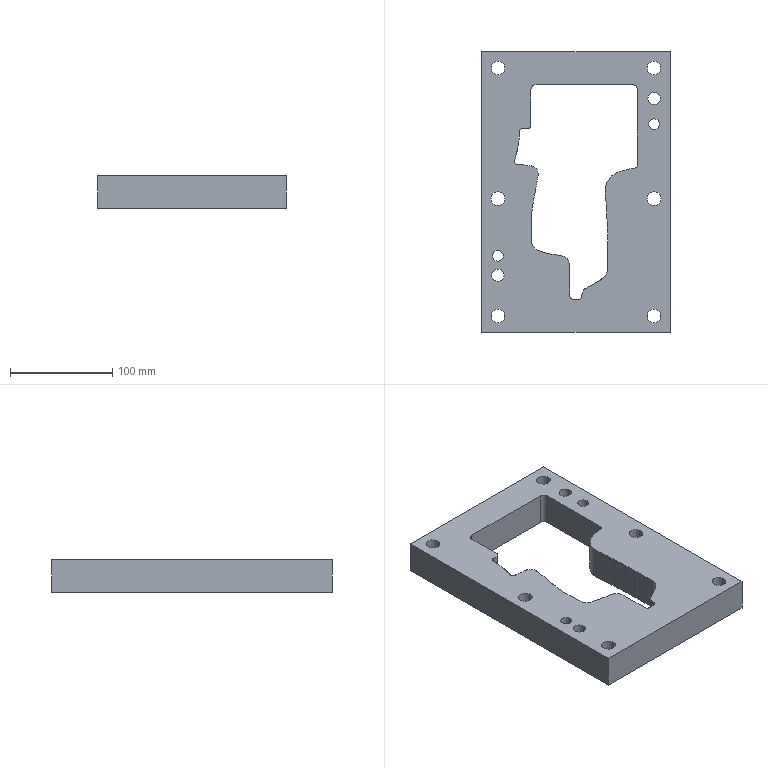Part | STEP file | lll_id3194_x_t | 1 solid | 104 faces | box 185 x 275 x 32 mm | volume 1049045 mm3 | cylinder 84 | plane 20 | commonest cylinder face diameters 6 x7 13.509 x6 20.008 x6 20 x3 10 x2 10.505 x2